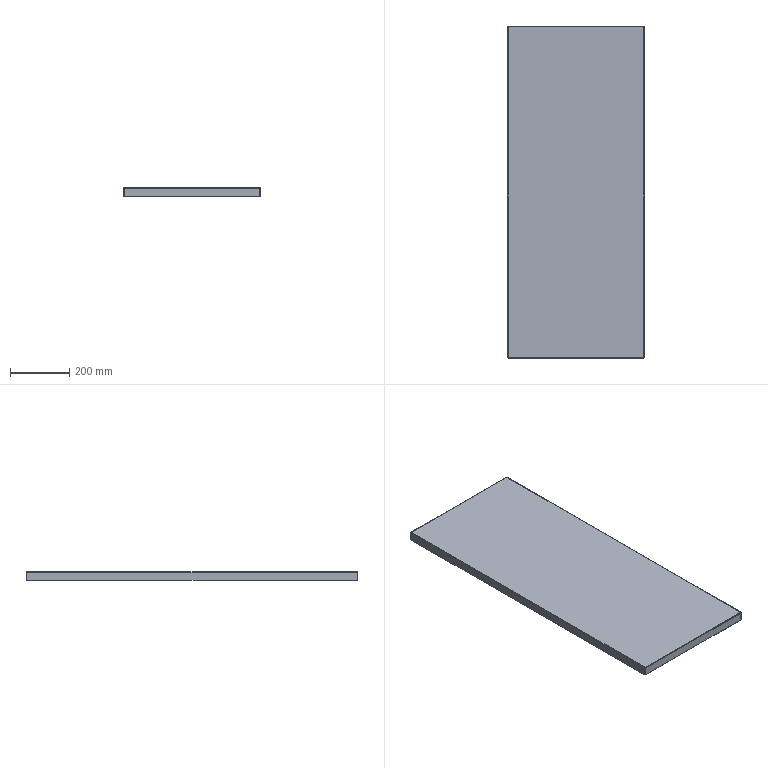Part | 1 solid | 38 faces | box 460 x 1120 x 30 mm | volume 724746 mm3 | plane 22 | spline 8 | cylinder 8 | commonest cylinder face diameters 1.465 x4 3.865 x4
STEP:
#1=CARTESIAN_POINT('',(-228.067,-558.067,-1.2));
#2=VERTEX_POINT('',#1);
#3=CARTESIAN_POINT('',(228.067,-558.067,-1.2));
#4=VERTEX_POINT('',#3);
#5=CARTESIAN_POINT('',(-228.093,-558.067,-1.2));
#6=DIRECTION('',(1.,0.,0.));
#7=VECTOR('',#6,1000.);
#8=LINE('',#5,#7);
#9=EDGE_CURVE('',#2,#4,#8,.T.);
#10=ORIENTED_EDGE('',*,*,#9,.F.);
#11=CARTESIAN_POINT('',(-228.067,558.067,-1.2));
#12=VERTEX_POINT('',#11);
#13=CARTESIAN_POINT('',(-228.067,558.093,-1.2));
#14=DIRECTION('',(0.,-1.,0.));
#15=VECTOR('',#14,1000.);
#16=LINE('',#13,#15);
#17=EDGE_CURVE('',#12,#2,#16,.T.);
#18=ORIENTED_EDGE('',*,*,#17,.F.);
#19=CARTESIAN_POINT('',(228.067,558.067,-1.2));
#20=VERTEX_POINT('',#19);
#21=CARTESIAN_POINT('',(228.093,558.067,-1.2));
#22=DIRECTION('',(-1.,0.,0.));
#23=VECTOR('',#22,1000.);
#24=LINE('',#21,#23);
#25=EDGE_CURVE('',#20,#12,#24,.T.);
#26=ORIENTED_EDGE('',*,*,#25,.F.);
#27=CARTESIAN_POINT('',(228.067,-558.093,-1.2));
#28=DIRECTION('',(0.,1.,0.));
#29=VECTOR('',#28,1000.);
#30=LINE('',#27,#29);
#31=EDGE_CURVE('',#4,#20,#30,.T.);
#32=ORIENTED_EDGE('',*,*,#31,.F.);
#33=EDGE_LOOP('',(#10,#18,#26,#32));
#34=FACE_OUTER_BOUND('',#33,.T.);
#35=CARTESIAN_POINT('',(0.,0.,-1.2));
#36=DIRECTION('',(0.,0.,1.));
#37=DIRECTION('',(1.,0.,0.));
#38=AXIS2_PLACEMENT_3D('',#35,#36,#37);
#39=PLANE('',#38);
#40=ADVANCED_FACE('',(#34),#39,.F.);
#41=CARTESIAN_POINT('',(-228.067,558.067,0.));
#42=VERTEX_POINT('',#41);
#43=CARTESIAN_POINT('',(-228.067,-558.067,0.));
#44=VERTEX_POINT('',#43);
#45=CARTESIAN_POINT('',(-228.067,558.093,0.));
#46=DIRECTION('',(0.,-1.,0.));
#47=VECTOR('',#46,1000.);
#48=LINE('',#45,#47);
#49=EDGE_CURVE('',#42,#44,#48,.T.);
#50=ORIENTED_EDGE('',*,*,#49,.T.);
#51=CARTESIAN_POINT('',(228.067,-558.067,0.));
#52=VERTEX_POINT('',#51);
#53=CARTESIAN_POINT('',(-228.093,-558.067,0.));
#54=DIRECTION('',(1.,0.,0.));
#55=VECTOR('',#54,1000.);
#56=LINE('',#53,#55);
#57=EDGE_CURVE('',#44,#52,#56,.T.);
#58=ORIENTED_EDGE('',*,*,#57,.T.);
#59=CARTESIAN_POINT('',(228.067,558.067,0.));
#60=VERTEX_POINT('',#59);
#61=CARTESIAN_POINT('',(228.067,-558.093,0.));
#62=DIRECTION('',(0.,1.,0.));
#63=VECTOR('',#62,1000.);
#64=LINE('',#61,#63);
#65=EDGE_CURVE('',#52,#60,#64,.T.);
#66=ORIENTED_EDGE('',*,*,#65,.T.);
#67=CARTESIAN_POINT('',(228.093,558.067,0.));
#68=DIRECTION('',(-1.,0.,0.));
#69=VECTOR('',#68,1000.);
#70=LINE('',#67,#69);
#71=EDGE_CURVE('',#60,#42,#70,.T.);
#72=ORIENTED_EDGE('',*,*,#71,.T.);
#73=EDGE_LOOP('',(#50,#58,#66,#72));
#74=FACE_OUTER_BOUND('',#73,.T.);
#75=CARTESIAN_POINT('',(0.,0.,0.));
#76=DIRECTION('',(0.,0.,1.));
#77=DIRECTION('',(1.,0.,0.));
#78=AXIS2_PLACEMENT_3D('',#75,#76,#77);
#79=PLANE('',#78);
#80=ADVANCED_FACE('',(#74),#79,.T.);
#81=CARTESIAN_POINT('',(-228.093,560.,-1.933));
#82=VERTEX_POINT('',#81);
#83=CARTESIAN_POINT('',(-228.093,558.8,-1.933));
#84=VERTEX_POINT('',#83);
#85=CARTESIAN_POINT('',(-228.093,558.8,-1.933));
#86=DIRECTION('',(0.,-1.,0.));
#87=VECTOR('',#86,1000.);
#88=LINE('',#85,#87);
#89=EDGE_CURVE('',#82,#84,#88,.T.);
#90=ORIENTED_EDGE('',*,*,#89,.T.);
#91=CARTESIAN_POINT('',(-228.067,558.067,-1.2));
#92=CARTESIAN_POINT('',(-228.072,558.259,-1.2));
#93=CARTESIAN_POINT('',(-228.076,558.45,-1.279));
#94=CARTESIAN_POINT('',(-228.084,558.721,-1.55));
#95=CARTESIAN_POINT('',(-228.089,558.8,-1.741));
#96=CARTESIAN_POINT('',(-228.093,558.8,-1.933));
#97=B_SPLINE_CURVE_WITH_KNOTS('',3,(#91,#92,#93,#94,#95,#96),.UNSPECIFIED.,.F.,.F.,(4,2,4),(0.,0.5,1.),.UNSPECIFIED.);
#98=EDGE_CURVE('',#12,#84,#97,.T.);
#99=ORIENTED_EDGE('',*,*,#98,.F.);
#100=CARTESIAN_POINT('',(-228.067,558.067,-1.2));
#101=DIRECTION('',(0.,0.,1.));
#102=VECTOR('',#101,1000.);
#103=LINE('',#100,#102);
#104=EDGE_CURVE('',#12,#42,#103,.T.);
#105=ORIENTED_EDGE('',*,*,#104,.T.);
#106=CARTESIAN_POINT('',(-228.067,558.067,0.));
#107=CARTESIAN_POINT('',(-228.07,558.32,0.));
#108=CARTESIAN_POINT('',(-228.072,558.573,-0.0503));
#109=CARTESIAN_POINT('',(-228.076,559.041,-0.2439));
#110=CARTESIAN_POINT('',(-228.078,559.255,-0.3872));
#111=CARTESIAN_POINT('',(-228.082,559.613,-0.7449));
#112=CARTESIAN_POINT('',(-228.084,559.756,-0.9593));
#113=CARTESIAN_POINT('',(-228.089,559.95,-1.427));
#114=CARTESIAN_POINT('',(-228.091,560.,-1.68));
#115=CARTESIAN_POINT('',(-228.093,560.,-1.933));
#116=B_SPLINE_CURVE_WITH_KNOTS('',3,(#106,#107,#108,#109,#110,#111,#112,#113,#114,#115),.UNSPECIFIED.,.F.,.F.,(4,2,2,2,4),(0.,0.25,0.5,0.75,1.),.UNSPECIFIED.);
#117=EDGE_CURVE('',#42,#82,#116,.T.);
#118=ORIENTED_EDGE('',*,*,#117,.T.);
#119=EDGE_LOOP('',(#90,#99,#105,#118));
#120=FACE_OUTER_BOUND('',#119,.T.);
#121=CARTESIAN_POINT('',(-228.067,558.067,0.012));
#122=CARTESIAN_POINT('',(-228.07,558.322,0.012));
#123=CARTESIAN_POINT('',(-228.072,558.576,-0.03861));
#124=CARTESIAN_POINT('',(-228.076,559.047,-0.2334));
#125=CARTESIAN_POINT('',(-228.078,559.262,-0.3776));
#126=CARTESIAN_POINT('',(-228.082,559.622,-0.7376));
#127=CARTESIAN_POINT('',(-228.084,559.767,-0.9533));
#128=CARTESIAN_POINT('',(-228.089,559.961,-1.424));
#129=CARTESIAN_POINT('',(-228.091,560.012,-1.678));
#130=CARTESIAN_POINT('',(-228.093,560.012,-1.933));
#131=CARTESIAN_POINT('',(-228.067,558.067,0.));
#132=CARTESIAN_POINT('',(-228.07,558.32,0.));
#133=CARTESIAN_POINT('',(-228.072,558.573,-0.0503));
#134=CARTESIAN_POINT('',(-228.076,559.041,-0.2439));
#135=CARTESIAN_POINT('',(-228.078,559.255,-0.3872));
#136=CARTESIAN_POINT('',(-228.082,559.613,-0.7449));
#137=CARTESIAN_POINT('',(-228.084,559.756,-0.9593));
#138=CARTESIAN_POINT('',(-228.089,559.95,-1.427));
#139=CARTESIAN_POINT('',(-228.091,560.,-1.68));
#140=CARTESIAN_POINT('',(-228.093,560.,-1.933));
#141=CARTESIAN_POINT('',(-228.067,558.067,-1.2));
#142=CARTESIAN_POINT('',(-228.07,558.163,-1.2));
#143=CARTESIAN_POINT('',(-228.072,558.259,-1.219));
#144=CARTESIAN_POINT('',(-228.076,558.436,-1.292));
#145=CARTESIAN_POINT('',(-228.078,558.518,-1.347));
#146=CARTESIAN_POINT('',(-228.082,558.653,-1.482));
#147=CARTESIAN_POINT('',(-228.084,558.708,-1.564));
#148=CARTESIAN_POINT('',(-228.089,558.781,-1.741));
#149=CARTESIAN_POINT('',(-228.091,558.8,-1.837));
#150=CARTESIAN_POINT('',(-228.093,558.8,-1.933));
#151=CARTESIAN_POINT('',(-228.067,558.067,-1.212));
#152=CARTESIAN_POINT('',(-228.07,558.162,-1.212));
#153=CARTESIAN_POINT('',(-228.072,558.256,-1.231));
#154=CARTESIAN_POINT('',(-228.076,558.43,-1.303));
#155=CARTESIAN_POINT('',(-228.078,558.51,-1.356));
#156=CARTESIAN_POINT('',(-228.082,558.644,-1.49));
#157=CARTESIAN_POINT('',(-228.084,558.697,-1.57));
#158=CARTESIAN_POINT('',(-228.089,558.769,-1.744));
#159=CARTESIAN_POINT('',(-228.091,558.788,-1.838));
#160=CARTESIAN_POINT('',(-228.093,558.788,-1.933));
#161=B_SPLINE_SURFACE_WITH_KNOTS('',1,3,((#121,#122,#123,#124,#125,#126,#127,#128,#129,#130),(#131,#132,#133,#134,#135,#136,#137,#138,#139,#140),(#141,#142,#143,#144,#145,#146,#147,#148,#149,#150),(#151,#152,#153,#154,#155,#156,#157,#158,#159,#160)),.UNSPECIFIED.,.F.,.F.,.F.,(2,1,1,2),(4,2,2,2,4),(-0.01,0.,1.,1.01),(0.,0.25,0.5,0.75,1.),.UNSPECIFIED.);
#162=ADVANCED_FACE('',(#120),#161,.F.);
#163=CARTESIAN_POINT('',(228.093,558.8,-1.933));
#164=VERTEX_POINT('',#163);
#165=CARTESIAN_POINT('',(228.093,558.8,-1.933));
#166=CARTESIAN_POINT('',(228.089,558.8,-1.741));
#167=CARTESIAN_POINT('',(228.084,558.721,-1.55));
#168=CARTESIAN_POINT('',(228.076,558.45,-1.279));
#169=CARTESIAN_POINT('',(228.072,558.259,-1.2));
#170=CARTESIAN_POINT('',(228.067,558.067,-1.2));
#171=B_SPLINE_CURVE_WITH_KNOTS('',3,(#165,#166,#167,#168,#169,#170),.UNSPECIFIED.,.F.,.F.,(4,2,4),(0.,0.5,1.),.UNSPECIFIED.);
#172=EDGE_CURVE('',#164,#20,#171,.T.);
#173=ORIENTED_EDGE('',*,*,#172,.F.);
#174=CARTESIAN_POINT('',(228.093,560.,-1.933));
#175=VERTEX_POINT('',#174);
#176=CARTESIAN_POINT('',(228.093,558.8,-1.933));
#177=DIRECTION('',(0.,-1.,0.));
#178=VECTOR('',#177,1000.);
#179=LINE('',#176,#178);
#180=EDGE_CURVE('',#175,#164,#179,.T.);
#181=ORIENTED_EDGE('',*,*,#180,.F.);
#182=CARTESIAN_POINT('',(228.093,560.,-1.933));
#183=CARTESIAN_POINT('',(228.091,560.,-1.68));
#184=CARTESIAN_POINT('',(228.089,559.95,-1.427));
#185=CARTESIAN_POINT('',(228.084,559.756,-0.9593));
#186=CARTESIAN_POINT('',(228.082,559.613,-0.7449));
#187=CARTESIAN_POINT('',(228.078,559.255,-0.3872));
#188=CARTESIAN_POINT('',(228.076,559.041,-0.2439));
#189=CARTESIAN_POINT('',(228.072,558.573,-0.0503));
#190=CARTESIAN_POINT('',(228.07,558.32,0.));
#191=CARTESIAN_POINT('',(228.067,558.067,0.));
#192=B_SPLINE_CURVE_WITH_KNOTS('',3,(#182,#183,#184,#185,#186,#187,#188,#189,#190,#191),.UNSPECIFIED.,.F.,.F.,(4,2,2,2,4),(0.,0.25,0.5,0.75,1.),.UNSPECIFIED.);
#193=EDGE_CURVE('',#175,#60,#192,.T.);
#194=ORIENTED_EDGE('',*,*,#193,.T.);
#195=CARTESIAN_POINT('',(228.067,558.067,-1.2));
#196=DIRECTION('',(0.,0.,1.));
#197=VECTOR('',#196,1000.);
#198=LINE('',#195,#197);
#199=EDGE_CURVE('',#20,#60,#198,.T.);
#200=ORIENTED_EDGE('',*,*,#199,.F.);
#201=EDGE_LOOP('',(#173,#181,#194,#200));
#202=FACE_OUTER_BOUND('',#201,.T.);
#203=CARTESIAN_POINT('',(228.093,560.012,-1.933));
#204=CARTESIAN_POINT('',(228.091,560.012,-1.678));
#205=CARTESIAN_POINT('',(228.089,559.961,-1.424));
#206=CARTESIAN_POINT('',(228.084,559.767,-0.9533));
#207=CARTESIAN_POINT('',(228.082,559.622,-0.7376));
#208=CARTESIAN_POINT('',(228.078,559.262,-0.3776));
#209=CARTESIAN_POINT('',(228.076,559.047,-0.2334));
#210=CARTESIAN_POINT('',(228.072,558.576,-0.03861));
#211=CARTESIAN_POINT('',(228.07,558.322,0.012));
#212=CARTESIAN_POINT('',(228.067,558.067,0.012));
#213=CARTESIAN_POINT('',(228.093,560.,-1.933));
#214=CARTESIAN_POINT('',(228.091,560.,-1.68));
#215=CARTESIAN_POINT('',(228.089,559.95,-1.427));
#216=CARTESIAN_POINT('',(228.084,559.756,-0.9593));
#217=CARTESIAN_POINT('',(228.082,559.613,-0.7449));
#218=CARTESIAN_POINT('',(228.078,559.255,-0.3872));
#219=CARTESIAN_POINT('',(228.076,559.041,-0.2439));
#220=CARTESIAN_POINT('',(228.072,558.573,-0.0503));
#221=CARTESIAN_POINT('',(228.07,558.32,0.));
#222=CARTESIAN_POINT('',(228.067,558.067,0.));
#223=CARTESIAN_POINT('',(228.093,558.8,-1.933));
#224=CARTESIAN_POINT('',(228.091,558.8,-1.837));
#225=CARTESIAN_POINT('',(228.089,558.781,-1.741));
#226=CARTESIAN_POINT('',(228.084,558.708,-1.564));
#227=CARTESIAN_POINT('',(228.082,558.653,-1.482));
#228=CARTESIAN_POINT('',(228.078,558.518,-1.347));
#229=CARTESIAN_POINT('',(228.076,558.436,-1.292));
#230=CARTESIAN_POINT('',(228.072,558.259,-1.219));
#231=CARTESIAN_POINT('',(228.07,558.163,-1.2));
#232=CARTESIAN_POINT('',(228.067,558.067,-1.2));
#233=CARTESIAN_POINT('',(228.093,558.788,-1.933));
#234=CARTESIAN_POINT('',(228.091,558.788,-1.838));
#235=CARTESIAN_POINT('',(228.089,558.769,-1.744));
#236=CARTESIAN_POINT('',(228.084,558.697,-1.57));
#237=CARTESIAN_POINT('',(228.082,558.644,-1.49));
#238=CARTESIAN_POINT('',(228.078,558.51,-1.356));
#239=CARTESIAN_POINT('',(228.076,558.43,-1.303));
#240=CARTESIAN_POINT('',(228.072,558.256,-1.231));
#241=CARTESIAN_POINT('',(228.07,558.162,-1.212));
#242=CARTESIAN_POINT('',(228.067,558.067,-1.212));
#243=B_SPLINE_SURFACE_WITH_KNOTS('',1,3,((#203,#204,#205,#206,#207,#208,#209,#210,#211,#212),(#213,#214,#215,#216,#217,#218,#219,#220,#221,#222),(#223,#224,#225,#226,#227,#228,#229,#230,#231,#232),(#233,#234,#235,#236,#237,#238,#239,#240,#241,#242)),.UNSPECIFIED.,.F.,.F.,.F.,(2,1,1,2),(4,2,2,2,4),(-0.01,0.,1.,1.01),(0.,0.25,0.5,0.75,1.),.UNSPECIFIED.);
#244=ADVANCED_FACE('',(#202),#243,.F.);
#245=ORIENTED_EDGE('',*,*,#71,.F.);
#246=ORIENTED_EDGE('',*,*,#193,.F.);
#247=CARTESIAN_POINT('',(0.,560.,-1.933));
#248=DIRECTION('',(1.,0.,0.));
#249=VECTOR('',#248,1000.);
#250=LINE('',#247,#249);
#251=EDGE_CURVE('',#82,#175,#250,.T.);
#252=ORIENTED_EDGE('',*,*,#251,.F.);
#253=ORIENTED_EDGE('',*,*,#117,.F.);
#254=EDGE_LOOP('',(#245,#246,#252,#253));
#255=FACE_OUTER_BOUND('',#254,.T.);
#256=CARTESIAN_POINT('',(228.093,558.067,-1.933));
#257=DIRECTION('',(1.,0.,0.));
#258=DIRECTION('',(0.,1.,0.));
#259=AXIS2_PLACEMENT_3D('',#256,#257,#258);
#260=CYLINDRICAL_SURFACE('',#259,1.933);
#261=ADVANCED_FACE('',(#255),#260,.T.);
#262=ORIENTED_EDGE('',*,*,#25,.T.);
#263=ORIENTED_EDGE('',*,*,#98,.T.);
#264=CARTESIAN_POINT('',(-230.,558.8,-1.933));
#265=DIRECTION('',(1.,0.,0.));
#266=VECTOR('',#265,1000.);
#267=LINE('',#264,#266);
#268=EDGE_CURVE('',#84,#164,#267,.T.);
#269=ORIENTED_EDGE('',*,*,#268,.T.);
#270=ORIENTED_EDGE('',*,*,#172,.T.);
#271=EDGE_LOOP('',(#262,#263,#269,#270));
#272=FACE_OUTER_BOUND('',#271,.T.);
#273=CARTESIAN_POINT('',(228.093,558.067,-1.933));
#274=DIRECTION('',(1.,0.,0.));
#275=DIRECTION('',(0.,1.,0.));
#276=AXIS2_PLACEMENT_3D('',#273,#274,#275);
#277=CYLINDRICAL_SURFACE('',#276,0.7326);
#278=ADVANCED_FACE('',(#272),#277,.F.);
#279=CARTESIAN_POINT('',(-228.093,558.8,-30.));
#280=VERTEX_POINT('',#279);
#281=CARTESIAN_POINT('',(-228.093,560.,-30.));
#282=VERTEX_POINT('',#281);
#283=CARTESIAN_POINT('',(-228.093,560.,-30.));
#284=DIRECTION('',(0.,1.,0.));
#285=VECTOR('',#284,1000.);
#286=LINE('',#283,#285);
#287=EDGE_CURVE('',#280,#282,#286,.T.);
#288=ORIENTED_EDGE('',*,*,#287,.F.);
#289=CARTESIAN_POINT('',(-228.093,558.8,0.));
#290=DIRECTION('',(0.,0.,-1.));
#291=VECTOR('',#290,1000.);
#292=LINE('',#289,#291);
#293=EDGE_CURVE('',#84,#280,#292,.T.);
#294=ORIENTED_EDGE('',*,*,#293,.F.);
#295=ORIENTED_EDGE('',*,*,#89,.F.);
#296=CARTESIAN_POINT('',(-228.093,560.,0.));
#297=DIRECTION('',(0.,0.,1.));
#298=VECTOR('',#297,1000.);
#299=LINE('',#296,#298);
#300=EDGE_CURVE('',#282,#82,#299,.T.);
#301=ORIENTED_EDGE('',*,*,#300,.F.);
#302=EDGE_LOOP('',(#288,#294,#295,#301));
#303=FACE_OUTER_BOUND('',#302,.T.);
#304=CARTESIAN_POINT('',(-228.093,558.8,-1.2));
#305=DIRECTION('',(-1.,0.,0.));
#306=DIRECTION('',(0.,0.,1.));
#307=AXIS2_PLACEMENT_3D('',#304,#305,#306);
#308=PLANE('',#307);
#309=ADVANCED_FACE('',(#303),#308,.T.);
#310=CARTESIAN_POINT('',(228.093,560.,-30.));
#311=VERTEX_POINT('',#310);
#312=CARTESIAN_POINT('',(228.093,560.,-1.2));
#313=DIRECTION('',(0.,0.,1.));
#314=VECTOR('',#313,1000.);
#315=LINE('',#312,#314);
#316=EDGE_CURVE('',#311,#175,#315,.T.);
#317=ORIENTED_EDGE('',*,*,#316,.F.);
#318=CARTESIAN_POINT('',(230.,560.,-30.));
#319=DIRECTION('',(1.,0.,0.));
#320=VECTOR('',#319,1000.);
#321=LINE('',#318,#320);
#322=EDGE_CURVE('',#282,#311,#321,.T.);
#323=ORIENTED_EDGE('',*,*,#322,.F.);
#324=ORIENTED_EDGE('',*,*,#300,.T.);
#325=ORIENTED_EDGE('',*,*,#251,.T.);
#326=EDGE_LOOP('',(#317,#323,#324,#325));
#327=FACE_OUTER_BOUND('',#326,.T.);
#328=CARTESIAN_POINT('',(0.,560.,0.));
#329=DIRECTION('',(0.,1.,0.));
#330=DIRECTION('',(0.,0.,-1.));
#331=AXIS2_PLACEMENT_3D('',#328,#329,#330);
#332=PLANE('',#331);
#333=ADVANCED_FACE('',(#327),#332,.T.);
#334=CARTESIAN_POINT('',(228.093,558.8,-30.));
#335=VERTEX_POINT('',#334);
#336=CARTESIAN_POINT('',(0.,558.8,-30.));
#337=DIRECTION('',(1.,0.,0.));
#338=VECTOR('',#337,1000.);
#339=LINE('',#336,#338);
#340=EDGE_CURVE('',#280,#335,#339,.T.);
#341=ORIENTED_EDGE('',*,*,#340,.T.);
#342=CARTESIAN_POINT('',(228.093,558.8,-1.2));
#343=DIRECTION('',(0.,0.,-1.));
#344=VECTOR('',#343,1000.);
#345=LINE('',#342,#344);
#346=EDGE_CURVE('',#164,#335,#345,.T.);
#347=ORIENTED_EDGE('',*,*,#346,.F.);
#348=ORIENTED_EDGE('',*,*,#268,.F.);
#349=ORIENTED_EDGE('',*,*,#293,.T.);
#350=EDGE_LOOP('',(#341,#347,#348,#349));
#351=FACE_OUTER_BOUND('',#350,.T.);
#352=CARTESIAN_POINT('',(0.,558.8,0.));
#353=DIRECTION('',(0.,1.,0.));
#354=DIRECTION('',(0.,0.,-1.));
#355=AXIS2_PLACEMENT_3D('',#352,#353,#354);
#356=PLANE('',#355);
#357=ADVANCED_FACE('',(#351),#356,.F.);
#358=CARTESIAN_POINT('',(228.093,558.8,-30.));
#359=DIRECTION('',(0.,1.,0.));
#360=VECTOR('',#359,1000.);
#361=LINE('',#358,#360);
#362=EDGE_CURVE('',#335,#311,#361,.T.);
#363=ORIENTED_EDGE('',*,*,#362,.F.);
#364=ORIENTED_EDGE('',*,*,#340,.F.);
#365=ORIENTED_EDGE('',*,*,#287,.T.);
#366=ORIENTED_EDGE('',*,*,#322,.T.);
#367=EDGE_LOOP('',(#363,#364,#365,#366));
#368=FACE_OUTER_BOUND('',#367,.T.);
#369=CARTESIAN_POINT('',(230.,560.,-30.));
#370=DIRECTION('',(0.,0.,-1.));
#371=DIRECTION('',(-1.,0.,0.));
#372=AXIS2_PLACEMENT_3D('',#369,#370,#371);
#373=PLANE('',#372);
#374=ADVANCED_FACE('',(#368),#373,.T.);
#375=ORIENTED_EDGE('',*,*,#346,.T.);
#376=ORIENTED_EDGE('',*,*,#362,.T.);
#377=ORIENTED_EDGE('',*,*,#316,.T.);
#378=ORIENTED_EDGE('',*,*,#180,.T.);
#379=EDGE_LOOP('',(#375,#376,#377,#378));
#380=FACE_OUTER_BOUND('',#379,.T.);
#381=CARTESIAN_POINT('',(228.093,558.8,-1.2));
#382=DIRECTION('',(-1.,0.,0.));
#383=DIRECTION('',(0.,0.,1.));
#384=AXIS2_PLACEMENT_3D('',#381,#382,#383);
#385=PLANE('',#384);
#386=ADVANCED_FACE('',(#380),#385,.F.);
#387=CARTESIAN_POINT('',(230.,558.093,-1.933));
#388=VERTEX_POINT('',#387);
#389=CARTESIAN_POINT('',(228.8,558.093,-1.933));
#390=VERTEX_POINT('',#389);
#391=CARTESIAN_POINT('',(228.8,558.093,-1.933));
#392=DIRECTION('',(-1.,0.,0.));
#393=VECTOR('',#392,1000.);
#394=LINE('',#391,#393);
#395=EDGE_CURVE('',#388,#390,#394,.T.);
#396=ORIENTED_EDGE('',*,*,#395,.T.);
#397=CARTESIAN_POINT('',(228.067,558.067,-1.2));
#398=CARTESIAN_POINT('',(228.259,558.072,-1.2));
#399=CARTESIAN_POINT('',(228.45,558.076,-1.279));
#400=CARTESIAN_POINT('',(228.721,558.084,-1.55));
#401=CARTESIAN_POINT('',(228.8,558.089,-1.741));
#402=CARTESIAN_POINT('',(228.8,558.093,-1.933));
#403=B_SPLINE_CURVE_WITH_KNOTS('',3,(#397,#398,#399,#400,#401,#402),.UNSPECIFIED.,.F.,.F.,(4,2,4),(0.,0.5,1.),.UNSPECIFIED.);
#404=EDGE_CURVE('',#20,#390,#403,.T.);
#405=ORIENTED_EDGE('',*,*,#404,.F.);
#406=ORIENTED_EDGE('',*,*,#199,.T.);
#407=CARTESIAN_POINT('',(228.067,558.067,0.));
#408=CARTESIAN_POINT('',(228.32,558.07,0.));
#409=CARTESIAN_POINT('',(228.573,558.072,-0.0503));
#410=CARTESIAN_POINT('',(229.041,558.076,-0.2439));
#411=CARTESIAN_POINT('',(229.255,558.078,-0.3872));
#412=CARTESIAN_POINT('',(229.613,558.082,-0.7449));
#413=CARTESIAN_POINT('',(229.756,558.084,-0.9593));
#414=CARTESIAN_POINT('',(229.95,558.089,-1.427));
#415=CARTESIAN_POINT('',(230.,558.091,-1.68));
#416=CARTESIAN_POINT('',(230.,558.093,-1.933));
#417=B_SPLINE_CURVE_WITH_KNOTS('',3,(#407,#408,#409,#410,#411,#412,#413,#414,#415,#416),.UNSPECIFIED.,.F.,.F.,(4,2,2,2,4),(0.,0.25,0.5,0.75,1.),.UNSPECIFIED.);
#418=EDGE_CURVE('',#60,#388,#417,.T.);
#419=ORIENTED_EDGE('',*,*,#418,.T.);
#420=EDGE_LOOP('',(#396,#405,#406,#419));
#421=FACE_OUTER_BOUND('',#420,.T.);
#422=CARTESIAN_POINT('',(228.067,558.067,0.012));
#423=CARTESIAN_POINT('',(228.322,558.07,0.012));
#424=CARTESIAN_POINT('',(228.576,558.072,-0.03861));
#425=CARTESIAN_POINT('',(229.047,558.076,-0.2334));
#426=CARTESIAN_POINT('',(229.262,558.078,-0.3776));
#427=CARTESIAN_POINT('',(229.622,558.082,-0.7376));
#428=CARTESIAN_POINT('',(229.767,558.084,-0.9533));
#429=CARTESIAN_POINT('',(229.961,558.089,-1.424));
#430=CARTESIAN_POINT('',(230.012,558.091,-1.678));
#431=CARTESIAN_POINT('',(230.012,558.093,-1.933));
#432=CARTESIAN_POINT('',(228.067,558.067,0.));
#433=CARTESIAN_POINT('',(228.32,558.07,0.));
#434=CARTESIAN_POINT('',(228.573,558.072,-0.0503));
#435=CARTESIAN_POINT('',(229.041,558.076,-0.2439));
#436=CARTESIAN_POINT('',(229.255,558.078,-0.3872));
#437=CARTESIAN_POINT('',(229.613,558.082,-0.7449));
#438=CARTESIAN_POINT('',(229.756,558.084,-0.9593));
#439=CARTESIAN_POINT('',(229.95,558.089,-1.427));
#440=CARTESIAN_POINT('',(230.,558.091,-1.68));
#441=CARTESIAN_POINT('',(230.,558.093,-1.933));
#442=CARTESIAN_POINT('',(228.067,558.067,-1.2));
#443=CARTESIAN_POINT('',(228.163,558.07,-1.2));
#444=CARTESIAN_POINT('',(228.259,558.072,-1.219));
#445=CARTESIAN_POINT('',(228.436,558.076,-1.292));
#446=CARTESIAN_POINT('',(228.518,558.078,-1.347));
#447=CARTESIAN_POINT('',(228.653,558.082,-1.482));
#448=CARTESIAN_POINT('',(228.708,558.084,-1.564));
#449=CARTESIAN_POINT('',(228.781,558.089,-1.741));
#450=CARTESIAN_POINT('',(228.8,558.091,-1.837));
#451=CARTESIAN_POINT('',(228.8,558.093,-1.933));
#452=CARTESIAN_POINT('',(228.067,558.067,-1.212));
#453=CARTESIAN_POINT('',(228.162,558.07,-1.212));
#454=CARTESIAN_POINT('',(228.256,558.072,-1.231));
#455=CARTESIAN_POINT('',(228.43,558.076,-1.303));
#456=CARTESIAN_POINT('',(228.51,558.078,-1.356));
#457=CARTESIAN_POINT('',(228.644,558.082,-1.49));
#458=CARTESIAN_POINT('',(228.697,558.084,-1.57));
#459=CARTESIAN_POINT('',(228.769,558.089,-1.744));
#460=CARTESIAN_POINT('',(228.788,558.091,-1.838));
#461=CARTESIAN_POINT('',(228.788,558.093,-1.933));
#462=B_SPLINE_SURFACE_WITH_KNOTS('',1,3,((#422,#423,#424,#425,#426,#427,#428,#429,#430,#431),(#432,#433,#434,#435,#436,#437,#438,#439,#440,#441),(#442,#443,#444,#445,#446,#447,#448,#449,#450,#451),(#452,#453,#454,#455,#456,#457,#458,#459,#460,#461)),.UNSPECIFIED.,.F.,.F.,.F.,(2,1,1,2),(4,2,2,2,4),(-0.01,0.,1.,1.01),(0.,0.25,0.5,0.75,1.),.UNSPECIFIED.);
#463=ADVANCED_FACE('',(#421),#462,.F.);
#464=CARTESIAN_POINT('',(228.8,-558.093,-1.933));
#465=VERTEX_POINT('',#464);
#466=CARTESIAN_POINT('',(228.8,-558.093,-1.933));
#467=CARTESIAN_POINT('',(228.8,-558.089,-1.741));
#468=CARTESIAN_POINT('',(228.721,-558.084,-1.55));
#469=CARTESIAN_POINT('',(228.45,-558.076,-1.279));
#470=CARTESIAN_POINT('',(228.259,-558.072,-1.2));
#471=CARTESIAN_POINT('',(228.067,-558.067,-1.2));
#472=B_SPLINE_CURVE_WITH_KNOTS('',3,(#466,#467,#468,#469,#470,#471),.UNSPECIFIED.,.F.,.F.,(4,2,4),(0.,0.5,1.),.UNSPECIFIED.);
#473=EDGE_CURVE('',#465,#4,#472,.T.);
#474=ORIENTED_EDGE('',*,*,#473,.F.);
#475=CARTESIAN_POINT('',(230.,-558.093,-1.933));
#476=VERTEX_POINT('',#475);
#477=CARTESIAN_POINT('',(228.8,-558.093,-1.933));
#478=DIRECTION('',(-1.,0.,0.));
#479=VECTOR('',#478,1000.);
#480=LINE('',#477,#479);
#481=EDGE_CURVE('',#476,#465,#480,.T.);
#482=ORIENTED_EDGE('',*,*,#481,.F.);
#483=CARTESIAN_POINT('',(230.,-558.093,-1.933));
#484=CARTESIAN_POINT('',(230.,-558.091,-1.68));
#485=CARTESIAN_POINT('',(229.95,-558.089,-1.427));
#486=CARTESIAN_POINT('',(229.756,-558.084,-0.9593));
#487=CARTESIAN_POINT('',(229.613,-558.082,-0.7449));
#488=CARTESIAN_POINT('',(229.255,-558.078,-0.3872));
#489=CARTESIAN_POINT('',(229.041,-558.076,-0.2439));
#490=CARTESIAN_POINT('',(228.573,-558.072,-0.0503));
#491=CARTESIAN_POINT('',(228.32,-558.07,0.));
#492=CARTESIAN_POINT('',(228.067,-558.067,0.));
#493=B_SPLINE_CURVE_WITH_KNOTS('',3,(#483,#484,#485,#486,#487,#488,#489,#490,#491,#492),.UNSPECIFIED.,.F.,.F.,(4,2,2,2,4),(0.,0.25,0.5,0.75,1.),.UNSPECIFIED.);
#494=EDGE_CURVE('',#476,#52,#493,.T.);
#495=ORIENTED_EDGE('',*,*,#494,.T.);
#496=CARTESIAN_POINT('',(228.067,-558.067,-1.2));
#497=DIRECTION('',(0.,0.,1.));
#498=VECTOR('',#497,1000.);
#499=LINE('',#496,#498);
#500=EDGE_CURVE('',#4,#52,#499,.T.);
#501=ORIENTED_EDGE('',*,*,#500,.F.);
#502=EDGE_LOOP('',(#474,#482,#495,#501));
#503=FACE_OUTER_BOUND('',#502,.T.);
#504=CARTESIAN_POINT('',(230.012,-558.093,-1.933));
#505=CARTESIAN_POINT('',(230.012,-558.091,-1.678));
#506=CARTESIAN_POINT('',(229.961,-558.089,-1.424));
#507=CARTESIAN_POINT('',(229.767,-558.084,-0.9533));
#508=CARTESIAN_POINT('',(229.622,-558.082,-0.7376));
#509=CARTESIAN_POINT('',(229.262,-558.078,-0.3776));
#510=CARTESIAN_POINT('',(229.047,-558.076,-0.2334));
#511=CARTESIAN_POINT('',(228.576,-558.072,-0.03861));
#512=CARTESIAN_POINT('',(228.322,-558.07,0.012));
#513=CARTESIAN_POINT('',(228.067,-558.067,0.012));
#514=CARTESIAN_POINT('',(230.,-558.093,-1.933));
#515=CARTESIAN_POINT('',(230.,-558.091,-1.68));
#516=CARTESIAN_POINT('',(229.95,-558.089,-1.427));
#517=CARTESIAN_POINT('',(229.756,-558.084,-0.9593));
#518=CARTESIAN_POINT('',(229.613,-558.082,-0.7449));
#519=CARTESIAN_POINT('',(229.255,-558.078,-0.3872));
#520=CARTESIAN_POINT('',(229.041,-558.076,-0.2439));
#521=CARTESIAN_POINT('',(228.573,-558.072,-0.0503));
#522=CARTESIAN_POINT('',(228.32,-558.07,0.));
#523=CARTESIAN_POINT('',(228.067,-558.067,0.));
#524=CARTESIAN_POINT('',(228.8,-558.093,-1.933));
#525=CARTESIAN_POINT('',(228.8,-558.091,-1.837));
#526=CARTESIAN_POINT('',(228.781,-558.089,-1.741));
#527=CARTESIAN_POINT('',(228.708,-558.084,-1.564));
#528=CARTESIAN_POINT('',(228.653,-558.082,-1.482));
#529=CARTESIAN_POINT('',(228.518,-558.078,-1.347));
#530=CARTESIAN_POINT('',(228.436,-558.076,-1.292));
#531=CARTESIAN_POINT('',(228.259,-558.072,-1.219));
#532=CARTESIAN_POINT('',(228.163,-558.07,-1.2));
#533=CARTESIAN_POINT('',(228.067,-558.067,-1.2));
#534=CARTESIAN_POINT('',(228.788,-558.093,-1.933));
#535=CARTESIAN_POINT('',(228.788,-558.091,-1.838));
#536=CARTESIAN_POINT('',(228.769,-558.089,-1.744));
#537=CARTESIAN_POINT('',(228.697,-558.084,-1.57));
#538=CARTESIAN_POINT('',(228.644,-558.082,-1.49));
#539=CARTESIAN_POINT('',(228.51,-558.078,-1.356));
#540=CARTESIAN_POINT('',(228.43,-558.076,-1.303));
#541=CARTESIAN_POINT('',(228.256,-558.072,-1.231));
#542=CARTESIAN_POINT('',(228.162,-558.07,-1.212));
#543=CARTESIAN_POINT('',(228.067,-558.067,-1.212));
#544=B_SPLINE_SURFACE_WITH_KNOTS('',1,3,((#504,#505,#506,#507,#508,#509,#510,#511,#512,#513),(#514,#515,#516,#517,#518,#519,#520,#521,#522,#523),(#524,#525,#526,#527,#528,#529,#530,#531,#532,#533),(#534,#535,#536,#537,#538,#539,#540,#541,#542,#543)),.UNSPECIFIED.,.F.,.F.,.F.,(2,1,1,2),(4,2,2,2,4),(-0.01,0.,1.,1.01),(0.,0.25,0.5,0.75,1.),.UNSPECIFIED.);
#545=ADVANCED_FACE('',(#503),#544,.F.);
#546=ORIENTED_EDGE('',*,*,#65,.F.);
#547=ORIENTED_EDGE('',*,*,#494,.F.);
#548=CARTESIAN_POINT('',(230.,560.,-1.933));
#549=DIRECTION('',(0.,1.,0.));
#550=VECTOR('',#549,1000.);
#551=LINE('',#548,#550);
#552=EDGE_CURVE('',#476,#388,#551,.T.);
#553=ORIENTED_EDGE('',*,*,#552,.T.);
#554=ORIENTED_EDGE('',*,*,#418,.F.);
#555=EDGE_LOOP('',(#546,#547,#553,#554));
#556=FACE_OUTER_BOUND('',#555,.T.);
#557=CARTESIAN_POINT('',(228.067,-558.093,-1.933));
#558=DIRECTION('',(0.,-1.,0.));
#559=DIRECTION('',(1.,0.,0.));
#560=AXIS2_PLACEMENT_3D('',#557,#558,#559);
#561=CYLINDRICAL_SURFACE('',#560,1.933);
#562=ADVANCED_FACE('',(#556),#561,.T.);
#563=ORIENTED_EDGE('',*,*,#31,.T.);
#564=ORIENTED_EDGE('',*,*,#404,.T.);
#565=CARTESIAN_POINT('',(228.8,560.,-1.933));
#566=DIRECTION('',(0.,-1.,0.));
#567=VECTOR('',#566,1000.);
#568=LINE('',#565,#567);
#569=EDGE_CURVE('',#390,#465,#568,.T.);
#570=ORIENTED_EDGE('',*,*,#569,.T.);
#571=ORIENTED_EDGE('',*,*,#473,.T.);
#572=EDGE_LOOP('',(#563,#564,#570,#571));
#573=FACE_OUTER_BOUND('',#572,.T.);
#574=CARTESIAN_POINT('',(228.067,-558.093,-1.933));
#575=DIRECTION('',(0.,-1.,0.));
#576=DIRECTION('',(1.,0.,0.));
#577=AXIS2_PLACEMENT_3D('',#574,#575,#576);
#578=CYLINDRICAL_SURFACE('',#577,0.7326);
#579=ADVANCED_FACE('',(#573),#578,.F.);
#580=CARTESIAN_POINT('',(228.8,558.093,-30.));
#581=VERTEX_POINT('',#580);
#582=CARTESIAN_POINT('',(230.,558.093,-30.));
#583=VERTEX_POINT('',#582);
#584=CARTESIAN_POINT('',(230.,558.093,-30.));
#585=DIRECTION('',(1.,0.,0.));
#586=VECTOR('',#585,1000.);
#587=LINE('',#584,#586);
#588=EDGE_CURVE('',#581,#583,#587,.T.);
#589=ORIENTED_EDGE('',*,*,#588,.F.);
#590=CARTESIAN_POINT('',(228.8,558.093,0.));
#591=DIRECTION('',(0.,0.,-1.));
#592=VECTOR('',#591,1000.);
#593=LINE('',#590,#592);
#594=EDGE_CURVE('',#390,#581,#593,.T.);
#595=ORIENTED_EDGE('',*,*,#594,.F.);
#596=ORIENTED_EDGE('',*,*,#395,.F.);
#597=CARTESIAN_POINT('',(230.,558.093,-1.2));
#598=DIRECTION('',(0.,0.,-1.));
#599=VECTOR('',#598,1000.);
#600=LINE('',#597,#599);
#601=EDGE_CURVE('',#388,#583,#600,.T.);
#602=ORIENTED_EDGE('',*,*,#601,.T.);
#603=EDGE_LOOP('',(#589,#595,#596,#602));
#604=FACE_OUTER_BOUND('',#603,.T.);
#605=CARTESIAN_POINT('',(228.8,558.093,-1.2));
#606=DIRECTION('',(0.,1.,0.));
#607=DIRECTION('',(0.,0.,-1.));
#608=AXIS2_PLACEMENT_3D('',#605,#606,#607);
#609=PLANE('',#608);
#610=ADVANCED_FACE('',(#604),#609,.T.);
#611=ORIENTED_EDGE('',*,*,#552,.F.);
#612=CARTESIAN_POINT('',(230.,-558.093,-30.));
#613=VERTEX_POINT('',#612);
#614=CARTESIAN_POINT('',(230.,-558.093,0.));
#615=DIRECTION('',(0.,0.,-1.));
#616=VECTOR('',#615,1000.);
#617=LINE('',#614,#616);
#618=EDGE_CURVE('',#476,#613,#617,.T.);
#619=ORIENTED_EDGE('',*,*,#618,.T.);
#620=CARTESIAN_POINT('',(230.,560.,-30.));
#621=DIRECTION('',(0.,-1.,0.));
#622=VECTOR('',#621,1000.);
#623=LINE('',#620,#622);
#624=EDGE_CURVE('',#583,#613,#623,.T.);
#625=ORIENTED_EDGE('',*,*,#624,.F.);
#626=ORIENTED_EDGE('',*,*,#601,.F.);
#627=EDGE_LOOP('',(#611,#619,#625,#626));
#628=FACE_OUTER_BOUND('',#627,.T.);
#629=CARTESIAN_POINT('',(230.,0.,0.));
#630=DIRECTION('',(-1.,0.,0.));
#631=DIRECTION('',(0.,0.,1.));
#632=AXIS2_PLACEMENT_3D('',#629,#630,#631);
#633=PLANE('',#632);
#634=ADVANCED_FACE('',(#628),#633,.F.);
#635=CARTESIAN_POINT('',(228.8,-558.093,-30.));
#636=VERTEX_POINT('',#635);
#637=CARTESIAN_POINT('',(228.8,-558.093,-1.2));
#638=DIRECTION('',(0.,0.,-1.));
#639=VECTOR('',#638,1000.);
#640=LINE('',#637,#639);
#641=EDGE_CURVE('',#465,#636,#640,.T.);
#642=ORIENTED_EDGE('',*,*,#641,.F.);
#643=ORIENTED_EDGE('',*,*,#569,.F.);
#644=ORIENTED_EDGE('',*,*,#594,.T.);
#645=CARTESIAN_POINT('',(228.8,0.,-30.));
#646=DIRECTION('',(0.,-1.,0.));
#647=VECTOR('',#646,1000.);
#648=LINE('',#645,#647);
#649=EDGE_CURVE('',#581,#636,#648,.T.);
#650=ORIENTED_EDGE('',*,*,#649,.T.);
#651=EDGE_LOOP('',(#642,#643,#644,#650));
#652=FACE_OUTER_BOUND('',#651,.T.);
#653=CARTESIAN_POINT('',(228.8,0.,0.));
#654=DIRECTION('',(-1.,0.,0.));
#655=DIRECTION('',(0.,0.,1.));
#656=AXIS2_PLACEMENT_3D('',#653,#654,#655);
#657=PLANE('',#656);
#658=ADVANCED_FACE('',(#652),#657,.T.);
#659=CARTESIAN_POINT('',(228.8,-558.093,-30.));
#660=DIRECTION('',(1.,0.,0.));
#661=VECTOR('',#660,1000.);
#662=LINE('',#659,#661);
#663=EDGE_CURVE('',#636,#613,#662,.T.);
#664=ORIENTED_EDGE('',*,*,#663,.F.);
#665=ORIENTED_EDGE('',*,*,#649,.F.);
#666=ORIENTED_EDGE('',*,*,#588,.T.);
#667=ORIENTED_EDGE('',*,*,#624,.T.);
#668=EDGE_LOOP('',(#664,#665,#666,#667));
#669=FACE_OUTER_BOUND('',#668,.T.);
#670=CARTESIAN_POINT('',(230.,560.,-30.));
#671=DIRECTION('',(0.,0.,-1.));
#672=DIRECTION('',(0.,-1.,0.));
#673=AXIS2_PLACEMENT_3D('',#670,#671,#672);
#674=PLANE('',#673);
#675=ADVANCED_FACE('',(#669),#674,.T.);
#676=ORIENTED_EDGE('',*,*,#641,.T.);
#677=ORIENTED_EDGE('',*,*,#663,.T.);
#678=ORIENTED_EDGE('',*,*,#618,.F.);
#679=ORIENTED_EDGE('',*,*,#481,.T.);
#680=EDGE_LOOP('',(#676,#677,#678,#679));
#681=FACE_OUTER_BOUND('',#680,.T.);
#682=CARTESIAN_POINT('',(228.8,-558.093,-1.2));
#683=DIRECTION('',(0.,1.,0.));
#684=DIRECTION('',(0.,0.,-1.));
#685=AXIS2_PLACEMENT_3D('',#682,#683,#684);
#686=PLANE('',#685);
#687=ADVANCED_FACE('',(#681),#686,.F.);
#688=CARTESIAN_POINT('',(-230.,-558.093,-1.933));
#689=VERTEX_POINT('',#688);
#690=CARTESIAN_POINT('',(-228.8,-558.093,-1.933));
#691=VERTEX_POINT('',#690);
#692=CARTESIAN_POINT('',(-228.8,-558.093,-1.933));
#693=DIRECTION('',(1.,0.,0.));
#694=VECTOR('',#693,1000.);
#695=LINE('',#692,#694);
#696=EDGE_CURVE('',#689,#691,#695,.T.);
#697=ORIENTED_EDGE('',*,*,#696,.T.);
#698=CARTESIAN_POINT('',(-228.067,-558.067,-1.2));
#699=CARTESIAN_POINT('',(-228.259,-558.072,-1.2));
#700=CARTESIAN_POINT('',(-228.45,-558.076,-1.279));
#701=CARTESIAN_POINT('',(-228.721,-558.084,-1.55));
#702=CARTESIAN_POINT('',(-228.8,-558.089,-1.741));
#703=CARTESIAN_POINT('',(-228.8,-558.093,-1.933));
#704=B_SPLINE_CURVE_WITH_KNOTS('',3,(#698,#699,#700,#701,#702,#703),.UNSPECIFIED.,.F.,.F.,(4,2,4),(0.,0.5,1.),.UNSPECIFIED.);
#705=EDGE_CURVE('',#2,#691,#704,.T.);
#706=ORIENTED_EDGE('',*,*,#705,.F.);
#707=CARTESIAN_POINT('',(-228.067,-558.067,-1.2));
#708=DIRECTION('',(0.,0.,1.));
#709=VECTOR('',#708,1000.);
#710=LINE('',#707,#709);
#711=EDGE_CURVE('',#2,#44,#710,.T.);
#712=ORIENTED_EDGE('',*,*,#711,.T.);
#713=CARTESIAN_POINT('',(-228.067,-558.067,0.));
#714=CARTESIAN_POINT('',(-228.32,-558.07,0.));
#715=CARTESIAN_POINT('',(-228.573,-558.072,-0.0503));
#716=CARTESIAN_POINT('',(-229.041,-558.076,-0.2439));
#717=CARTESIAN_POINT('',(-229.255,-558.078,-0.3872));
#718=CARTESIAN_POINT('',(-229.613,-558.082,-0.7449));
#719=CARTESIAN_POINT('',(-229.756,-558.084,-0.9593));
#720=CARTESIAN_POINT('',(-229.95,-558.089,-1.427));
#721=CARTESIAN_POINT('',(-230.,-558.091,-1.68));
#722=CARTESIAN_POINT('',(-230.,-558.093,-1.933));
#723=B_SPLINE_CURVE_WITH_KNOTS('',3,(#713,#714,#715,#716,#717,#718,#719,#720,#721,#722),.UNSPECIFIED.,.F.,.F.,(4,2,2,2,4),(0.,0.25,0.5,0.75,1.),.UNSPECIFIED.);
#724=EDGE_CURVE('',#44,#689,#723,.T.);
#725=ORIENTED_EDGE('',*,*,#724,.T.);
#726=EDGE_LOOP('',(#697,#706,#712,#725));
#727=FACE_OUTER_BOUND('',#726,.T.);
#728=CARTESIAN_POINT('',(-228.067,-558.067,0.012));
#729=CARTESIAN_POINT('',(-228.322,-558.07,0.012));
#730=CARTESIAN_POINT('',(-228.576,-558.072,-0.03861));
#731=CARTESIAN_POINT('',(-229.047,-558.076,-0.2334));
#732=CARTESIAN_POINT('',(-229.262,-558.078,-0.3776));
#733=CARTESIAN_POINT('',(-229.622,-558.082,-0.7376));
#734=CARTESIAN_POINT('',(-229.767,-558.084,-0.9533));
#735=CARTESIAN_POINT('',(-229.961,-558.089,-1.424));
#736=CARTESIAN_POINT('',(-230.012,-558.091,-1.678));
#737=CARTESIAN_POINT('',(-230.012,-558.093,-1.933));
#738=CARTESIAN_POINT('',(-228.067,-558.067,0.));
#739=CARTESIAN_POINT('',(-228.32,-558.07,0.));
#740=CARTESIAN_POINT('',(-228.573,-558.072,-0.0503));
#741=CARTESIAN_POINT('',(-229.041,-558.076,-0.2439));
#742=CARTESIAN_POINT('',(-229.255,-558.078,-0.3872));
#743=CARTESIAN_POINT('',(-229.613,-558.082,-0.7449));
#744=CARTESIAN_POINT('',(-229.756,-558.084,-0.9593));
#745=CARTESIAN_POINT('',(-229.95,-558.089,-1.427));
#746=CARTESIAN_POINT('',(-230.,-558.091,-1.68));
#747=CARTESIAN_POINT('',(-230.,-558.093,-1.933));
#748=CARTESIAN_POINT('',(-228.067,-558.067,-1.2));
#749=CARTESIAN_POINT('',(-228.163,-558.07,-1.2));
#750=CARTESIAN_POINT('',(-228.259,-558.072,-1.219));
#751=CARTESIAN_POINT('',(-228.436,-558.076,-1.292));
#752=CARTESIAN_POINT('',(-228.518,-558.078,-1.347));
#753=CARTESIAN_POINT('',(-228.653,-558.082,-1.482));
#754=CARTESIAN_POINT('',(-228.708,-558.084,-1.564));
#755=CARTESIAN_POINT('',(-228.781,-558.089,-1.741));
#756=CARTESIAN_POINT('',(-228.8,-558.091,-1.837));
#757=CARTESIAN_POINT('',(-228.8,-558.093,-1.933));
#758=CARTESIAN_POINT('',(-228.067,-558.067,-1.212));
#759=CARTESIAN_POINT('',(-228.162,-558.07,-1.212));
#760=CARTESIAN_POINT('',(-228.256,-558.072,-1.231));
#761=CARTESIAN_POINT('',(-228.43,-558.076,-1.303));
#762=CARTESIAN_POINT('',(-228.51,-558.078,-1.356));
#763=CARTESIAN_POINT('',(-228.644,-558.082,-1.49));
#764=CARTESIAN_POINT('',(-228.697,-558.084,-1.57));
#765=CARTESIAN_POINT('',(-228.769,-558.089,-1.744));
#766=CARTESIAN_POINT('',(-228.788,-558.091,-1.838));
#767=CARTESIAN_POINT('',(-228.788,-558.093,-1.933));
#768=B_SPLINE_SURFACE_WITH_KNOTS('',1,3,((#728,#729,#730,#731,#732,#733,#734,#735,#736,#737),(#738,#739,#740,#741,#742,#743,#744,#745,#746,#747),(#748,#749,#750,#751,#752,#753,#754,#755,#756,#757),(#758,#759,#760,#761,#762,#763,#764,#765,#766,#767)),.UNSPECIFIED.,.F.,.F.,.F.,(2,1,1,2),(4,2,2,2,4),(-0.01,0.,1.,1.01),(0.,0.25,0.5,0.75,1.),.UNSPECIFIED.);
#769=ADVANCED_FACE('',(#727),#768,.F.);
#770=CARTESIAN_POINT('',(-228.8,558.093,-1.933));
#771=VERTEX_POINT('',#770);
#772=CARTESIAN_POINT('',(-228.8,558.093,-1.933));
#773=CARTESIAN_POINT('',(-228.8,558.089,-1.741));
#774=CARTESIAN_POINT('',(-228.721,558.084,-1.55));
#775=CARTESIAN_POINT('',(-228.45,558.076,-1.279));
#776=CARTESIAN_POINT('',(-228.259,558.072,-1.2));
#777=CARTESIAN_POINT('',(-228.067,558.067,-1.2));
#778=B_SPLINE_CURVE_WITH_KNOTS('',3,(#772,#773,#774,#775,#776,#777),.UNSPECIFIED.,.F.,.F.,(4,2,4),(0.,0.5,1.),.UNSPECIFIED.);
#779=EDGE_CURVE('',#771,#12,#778,.T.);
#780=ORIENTED_EDGE('',*,*,#779,.F.);
#781=CARTESIAN_POINT('',(-230.,558.093,-1.933));
#782=VERTEX_POINT('',#781);
#783=CARTESIAN_POINT('',(-228.8,558.093,-1.933));
#784=DIRECTION('',(1.,0.,0.));
#785=VECTOR('',#784,1000.);
#786=LINE('',#783,#785);
#787=EDGE_CURVE('',#782,#771,#786,.T.);
#788=ORIENTED_EDGE('',*,*,#787,.F.);
#789=CARTESIAN_POINT('',(-230.,558.093,-1.933));
#790=CARTESIAN_POINT('',(-230.,558.091,-1.68));
#791=CARTESIAN_POINT('',(-229.95,558.089,-1.427));
#792=CARTESIAN_POINT('',(-229.756,558.084,-0.9593));
#793=CARTESIAN_POINT('',(-229.613,558.082,-0.7449));
#794=CARTESIAN_POINT('',(-229.255,558.078,-0.3872));
#795=CARTESIAN_POINT('',(-229.041,558.076,-0.2439));
#796=CARTESIAN_POINT('',(-228.573,558.072,-0.0503));
#797=CARTESIAN_POINT('',(-228.32,558.07,0.));
#798=CARTESIAN_POINT('',(-228.067,558.067,0.));
#799=B_SPLINE_CURVE_WITH_KNOTS('',3,(#789,#790,#791,#792,#793,#794,#795,#796,#797,#798),.UNSPECIFIED.,.F.,.F.,(4,2,2,2,4),(0.,0.25,0.5,0.75,1.),.UNSPECIFIED.);
#800=EDGE_CURVE('',#782,#42,#799,.T.);
#801=ORIENTED_EDGE('',*,*,#800,.T.);
#802=ORIENTED_EDGE('',*,*,#104,.F.);
#803=EDGE_LOOP('',(#780,#788,#801,#802));
#804=FACE_OUTER_BOUND('',#803,.T.);
#805=CARTESIAN_POINT('',(-230.012,558.093,-1.933));
#806=CARTESIAN_POINT('',(-230.012,558.091,-1.678));
#807=CARTESIAN_POINT('',(-229.961,558.089,-1.424));
#808=CARTESIAN_POINT('',(-229.767,558.084,-0.9533));
#809=CARTESIAN_POINT('',(-229.622,558.082,-0.7376));
#810=CARTESIAN_POINT('',(-229.262,558.078,-0.3776));
#811=CARTESIAN_POINT('',(-229.047,558.076,-0.2334));
#812=CARTESIAN_POINT('',(-228.576,558.072,-0.03861));
#813=CARTESIAN_POINT('',(-228.322,558.07,0.012));
#814=CARTESIAN_POINT('',(-228.067,558.067,0.012));
#815=CARTESIAN_POINT('',(-230.,558.093,-1.933));
#816=CARTESIAN_POINT('',(-230.,558.091,-1.68));
#817=CARTESIAN_POINT('',(-229.95,558.089,-1.427));
#818=CARTESIAN_POINT('',(-229.756,558.084,-0.9593));
#819=CARTESIAN_POINT('',(-229.613,558.082,-0.7449));
#820=CARTESIAN_POINT('',(-229.255,558.078,-0.3872));
#821=CARTESIAN_POINT('',(-229.041,558.076,-0.2439));
#822=CARTESIAN_POINT('',(-228.573,558.072,-0.0503));
#823=CARTESIAN_POINT('',(-228.32,558.07,0.));
#824=CARTESIAN_POINT('',(-228.067,558.067,0.));
#825=CARTESIAN_POINT('',(-228.8,558.093,-1.933));
#826=CARTESIAN_POINT('',(-228.8,558.091,-1.837));
#827=CARTESIAN_POINT('',(-228.781,558.089,-1.741));
#828=CARTESIAN_POINT('',(-228.708,558.084,-1.564));
#829=CARTESIAN_POINT('',(-228.653,558.082,-1.482));
#830=CARTESIAN_POINT('',(-228.518,558.078,-1.347));
#831=CARTESIAN_POINT('',(-228.436,558.076,-1.292));
#832=CARTESIAN_POINT('',(-228.259,558.072,-1.219));
#833=CARTESIAN_POINT('',(-228.163,558.07,-1.2));
#834=CARTESIAN_POINT('',(-228.067,558.067,-1.2));
#835=CARTESIAN_POINT('',(-228.788,558.093,-1.933));
#836=CARTESIAN_POINT('',(-228.788,558.091,-1.838));
#837=CARTESIAN_POINT('',(-228.769,558.089,-1.744));
#838=CARTESIAN_POINT('',(-228.697,558.084,-1.57));
#839=CARTESIAN_POINT('',(-228.644,558.082,-1.49));
#840=CARTESIAN_POINT('',(-228.51,558.078,-1.356));
#841=CARTESIAN_POINT('',(-228.43,558.076,-1.303));
#842=CARTESIAN_POINT('',(-228.256,558.072,-1.231));
#843=CARTESIAN_POINT('',(-228.162,558.07,-1.212));
#844=CARTESIAN_POINT('',(-228.067,558.067,-1.212));
#845=B_SPLINE_SURFACE_WITH_KNOTS('',1,3,((#805,#806,#807,#808,#809,#810,#811,#812,#813,#814),(#815,#816,#817,#818,#819,#820,#821,#822,#823,#824),(#825,#826,#827,#828,#829,#830,#831,#832,#833,#834),(#835,#836,#837,#838,#839,#840,#841,#842,#843,#844)),.UNSPECIFIED.,.F.,.F.,.F.,(2,1,1,2),(4,2,2,2,4),(-0.01,0.,1.,1.01),(0.,0.25,0.5,0.75,1.),.UNSPECIFIED.);
#846=ADVANCED_FACE('',(#804),#845,.F.);
#847=ORIENTED_EDGE('',*,*,#49,.F.);
#848=ORIENTED_EDGE('',*,*,#800,.F.);
#849=CARTESIAN_POINT('',(-230.,-560.,-1.933));
#850=DIRECTION('',(0.,-1.,0.));
#851=VECTOR('',#850,1000.);
#852=LINE('',#849,#851);
#853=EDGE_CURVE('',#782,#689,#852,.T.);
#854=ORIENTED_EDGE('',*,*,#853,.T.);
#855=ORIENTED_EDGE('',*,*,#724,.F.);
#856=EDGE_LOOP('',(#847,#848,#854,#855));
#857=FACE_OUTER_BOUND('',#856,.T.);
#858=CARTESIAN_POINT('',(-228.067,558.093,-1.933));
#859=DIRECTION('',(0.,1.,0.));
#860=DIRECTION('',(-1.,0.,0.));
#861=AXIS2_PLACEMENT_3D('',#858,#859,#860);
#862=CYLINDRICAL_SURFACE('',#861,1.933);
#863=ADVANCED_FACE('',(#857),#862,.T.);
#864=ORIENTED_EDGE('',*,*,#17,.T.);
#865=ORIENTED_EDGE('',*,*,#705,.T.);
#866=CARTESIAN_POINT('',(-228.8,-560.,-1.933));
#867=DIRECTION('',(0.,1.,0.));
#868=VECTOR('',#867,1000.);
#869=LINE('',#866,#868);
#870=EDGE_CURVE('',#691,#771,#869,.T.);
#871=ORIENTED_EDGE('',*,*,#870,.T.);
#872=ORIENTED_EDGE('',*,*,#779,.T.);
#873=EDGE_LOOP('',(#864,#865,#871,#872));
#874=FACE_OUTER_BOUND('',#873,.T.);
#875=CARTESIAN_POINT('',(-228.067,558.093,-1.933));
#876=DIRECTION('',(0.,1.,0.));
#877=DIRECTION('',(-1.,0.,0.));
#878=AXIS2_PLACEMENT_3D('',#875,#876,#877);
#879=CYLINDRICAL_SURFACE('',#878,0.7326);
#880=ADVANCED_FACE('',(#874),#879,.F.);
#881=CARTESIAN_POINT('',(-228.8,-558.093,-30.));
#882=VERTEX_POINT('',#881);
#883=CARTESIAN_POINT('',(-230.,-558.093,-30.));
#884=VERTEX_POINT('',#883);
#885=CARTESIAN_POINT('',(-230.,-558.093,-30.));
#886=DIRECTION('',(-1.,0.,0.));
#887=VECTOR('',#886,1000.);
#888=LINE('',#885,#887);
#889=EDGE_CURVE('',#882,#884,#888,.T.);
#890=ORIENTED_EDGE('',*,*,#889,.F.);
#891=CARTESIAN_POINT('',(-228.8,-558.093,0.));
#892=DIRECTION('',(0.,0.,-1.));
#893=VECTOR('',#892,1000.);
#894=LINE('',#891,#893);
#895=EDGE_CURVE('',#691,#882,#894,.T.);
#896=ORIENTED_EDGE('',*,*,#895,.F.);
#897=ORIENTED_EDGE('',*,*,#696,.F.);
#898=CARTESIAN_POINT('',(-230.,-558.093,-1.2));
#899=DIRECTION('',(0.,0.,-1.));
#900=VECTOR('',#899,1000.);
#901=LINE('',#898,#900);
#902=EDGE_CURVE('',#689,#884,#901,.T.);
#903=ORIENTED_EDGE('',*,*,#902,.T.);
#904=EDGE_LOOP('',(#890,#896,#897,#903));
#905=FACE_OUTER_BOUND('',#904,.T.);
#906=CARTESIAN_POINT('',(-228.8,-558.093,-1.2));
#907=DIRECTION('',(0.,-1.,0.));
#908=DIRECTION('',(0.,0.,-1.));
#909=AXIS2_PLACEMENT_3D('',#906,#907,#908);
#910=PLANE('',#909);
#911=ADVANCED_FACE('',(#905),#910,.T.);
#912=ORIENTED_EDGE('',*,*,#853,.F.);
#913=CARTESIAN_POINT('',(-230.,558.093,-30.));
#914=VERTEX_POINT('',#913);
#915=CARTESIAN_POINT('',(-230.,558.093,0.));
#916=DIRECTION('',(0.,0.,-1.));
#917=VECTOR('',#916,1000.);
#918=LINE('',#915,#917);
#919=EDGE_CURVE('',#782,#914,#918,.T.);
#920=ORIENTED_EDGE('',*,*,#919,.T.);
#921=CARTESIAN_POINT('',(-230.,-560.,-30.));
#922=DIRECTION('',(0.,1.,0.));
#923=VECTOR('',#922,1000.);
#924=LINE('',#921,#923);
#925=EDGE_CURVE('',#884,#914,#924,.T.);
#926=ORIENTED_EDGE('',*,*,#925,.F.);
#927=ORIENTED_EDGE('',*,*,#902,.F.);
#928=EDGE_LOOP('',(#912,#920,#926,#927));
#929=FACE_OUTER_BOUND('',#928,.T.);
#930=CARTESIAN_POINT('',(-230.,0.,0.));
#931=DIRECTION('',(1.,0.,0.));
#932=DIRECTION('',(0.,0.,-1.));
#933=AXIS2_PLACEMENT_3D('',#930,#931,#932);
#934=PLANE('',#933);
#935=ADVANCED_FACE('',(#929),#934,.F.);
#936=CARTESIAN_POINT('',(-228.8,558.093,-30.));
#937=VERTEX_POINT('',#936);
#938=CARTESIAN_POINT('',(-228.8,558.093,-1.2));
#939=DIRECTION('',(0.,0.,-1.));
#940=VECTOR('',#939,1000.);
#941=LINE('',#938,#940);
#942=EDGE_CURVE('',#771,#937,#941,.T.);
#943=ORIENTED_EDGE('',*,*,#942,.F.);
#944=ORIENTED_EDGE('',*,*,#870,.F.);
#945=ORIENTED_EDGE('',*,*,#895,.T.);
#946=CARTESIAN_POINT('',(-228.8,0.,-30.));
#947=DIRECTION('',(0.,1.,0.));
#948=VECTOR('',#947,1000.);
#949=LINE('',#946,#948);
#950=EDGE_CURVE('',#882,#937,#949,.T.);
#951=ORIENTED_EDGE('',*,*,#950,.T.);
#952=EDGE_LOOP('',(#943,#944,#945,#951));
#953=FACE_OUTER_BOUND('',#952,.T.);
#954=CARTESIAN_POINT('',(-228.8,0.,0.));
#955=DIRECTION('',(1.,0.,0.));
#956=DIRECTION('',(0.,0.,-1.));
#957=AXIS2_PLACEMENT_3D('',#954,#955,#956);
#958=PLANE('',#957);
#959=ADVANCED_FACE('',(#953),#958,.T.);
#960=CARTESIAN_POINT('',(-228.8,558.093,-30.));
#961=DIRECTION('',(-1.,0.,0.));
#962=VECTOR('',#961,1000.);
#963=LINE('',#960,#962);
#964=EDGE_CURVE('',#937,#914,#963,.T.);
#965=ORIENTED_EDGE('',*,*,#964,.F.);
#966=ORIENTED_EDGE('',*,*,#950,.F.);
#967=ORIENTED_EDGE('',*,*,#889,.T.);
#968=ORIENTED_EDGE('',*,*,#925,.T.);
#969=EDGE_LOOP('',(#965,#966,#967,#968));
#970=FACE_OUTER_BOUND('',#969,.T.);
#971=CARTESIAN_POINT('',(-230.,-560.,-30.));
#972=DIRECTION('',(0.,0.,-1.));
#973=DIRECTION('',(-1.,0.,0.));
#974=AXIS2_PLACEMENT_3D('',#971,#972,#973);
#975=PLANE('',#974);
#976=ADVANCED_FACE('',(#970),#975,.T.);
#977=ORIENTED_EDGE('',*,*,#942,.T.);
#978=ORIENTED_EDGE('',*,*,#964,.T.);
#979=ORIENTED_EDGE('',*,*,#919,.F.);
#980=ORIENTED_EDGE('',*,*,#787,.T.);
#981=EDGE_LOOP('',(#977,#978,#979,#980));
#982=FACE_OUTER_BOUND('',#981,.T.);
#983=CARTESIAN_POINT('',(-228.8,558.093,-1.2));
#984=DIRECTION('',(0.,-1.,0.));
#985=DIRECTION('',(0.,0.,-1.));
#986=AXIS2_PLACEMENT_3D('',#983,#984,#985);
#987=PLANE('',#986);
#988=ADVANCED_FACE('',(#982),#987,.F.);
#989=CARTESIAN_POINT('',(228.093,-560.,-1.933));
#990=VERTEX_POINT('',#989);
#991=CARTESIAN_POINT('',(228.093,-558.8,-1.933));
#992=VERTEX_POINT('',#991);
#993=CARTESIAN_POINT('',(228.093,-558.8,-1.933));
#994=DIRECTION('',(0.,1.,0.));
#995=VECTOR('',#994,1000.);
#996=LINE('',#993,#995);
#997=EDGE_CURVE('',#990,#992,#996,.T.);
#998=ORIENTED_EDGE('',*,*,#997,.T.);
#999=CARTESIAN_POINT('',(228.067,-558.067,-1.2));
#1000=CARTESIAN_POINT('',(228.072,-558.259,-1.2));
#1001=CARTESIAN_POINT('',(228.076,-558.45,-1.279));
#1002=CARTESIAN_POINT('',(228.084,-558.721,-1.55));
#1003=CARTESIAN_POINT('',(228.089,-558.8,-1.741));
#1004=CARTESIAN_POINT('',(228.093,-558.8,-1.933));
#1005=B_SPLINE_CURVE_WITH_KNOTS('',3,(#999,#1000,#1001,#1002,#1003,#1004),.UNSPECIFIED.,.F.,.F.,(4,2,4),(0.,0.5,1.),.UNSPECIFIED.);
#1006=EDGE_CURVE('',#4,#992,#1005,.T.);
#1007=ORIENTED_EDGE('',*,*,#1006,.F.);
#1008=ORIENTED_EDGE('',*,*,#500,.T.);
#1009=CARTESIAN_POINT('',(228.067,-558.067,0.));
#1010=CARTESIAN_POINT('',(228.07,-558.32,0.));
#1011=CARTESIAN_POINT('',(228.072,-558.573,-0.0503));
#1012=CARTESIAN_POINT('',(228.076,-559.041,-0.2439));
#1013=CARTESIAN_POINT('',(228.078,-559.255,-0.3872));
#1014=CARTESIAN_POINT('',(228.082,-559.613,-0.7449));
#1015=CARTESIAN_POINT('',(228.084,-559.756,-0.9593));
#1016=CARTESIAN_POINT('',(228.089,-559.95,-1.427));
#1017=CARTESIAN_POINT('',(228.091,-560.,-1.68));
#1018=CARTESIAN_POINT('',(228.093,-560.,-1.933));
#1019=B_SPLINE_CURVE_WITH_KNOTS('',3,(#1009,#1010,#1011,#1012,#1013,#1014,#1015,#1016,#1017,#1018),.UNSPECIFIED.,.F.,.F.,(4,2,2,2,4),(0.,0.25,0.5,0.75,1.),.UNSPECIFIED.);
#1020=EDGE_CURVE('',#52,#990,#1019,.T.);
#1021=ORIENTED_EDGE('',*,*,#1020,.T.);
#1022=EDGE_LOOP('',(#998,#1007,#1008,#1021));
#1023=FACE_OUTER_BOUND('',#1022,.T.);
#1024=CARTESIAN_POINT('',(228.067,-558.067,0.012));
#1025=CARTESIAN_POINT('',(228.07,-558.322,0.012));
#1026=CARTESIAN_POINT('',(228.072,-558.576,-0.03861));
#1027=CARTESIAN_POINT('',(228.076,-559.047,-0.2334));
#1028=CARTESIAN_POINT('',(228.078,-559.262,-0.3776));
#1029=CARTESIAN_POINT('',(228.082,-559.622,-0.7376));
#1030=CARTESIAN_POINT('',(228.084,-559.767,-0.9533));
#1031=CARTESIAN_POINT('',(228.089,-559.961,-1.424));
#1032=CARTESIAN_POINT('',(228.091,-560.012,-1.678));
#1033=CARTESIAN_POINT('',(228.093,-560.012,-1.933));
#1034=CARTESIAN_POINT('',(228.067,-558.067,0.));
#1035=CARTESIAN_POINT('',(228.07,-558.32,0.));
#1036=CARTESIAN_POINT('',(228.072,-558.573,-0.0503));
#1037=CARTESIAN_POINT('',(228.076,-559.041,-0.2439));
#1038=CARTESIAN_POINT('',(228.078,-559.255,-0.3872));
#1039=CARTESIAN_POINT('',(228.082,-559.613,-0.7449));
#1040=CARTESIAN_POINT('',(228.084,-559.756,-0.9593));
#1041=CARTESIAN_POINT('',(228.089,-559.95,-1.427));
#1042=CARTESIAN_POINT('',(228.091,-560.,-1.68));
#1043=CARTESIAN_POINT('',(228.093,-560.,-1.933));
#1044=CARTESIAN_POINT('',(228.067,-558.067,-1.2));
#1045=CARTESIAN_POINT('',(228.07,-558.163,-1.2));
#1046=CARTESIAN_POINT('',(228.072,-558.259,-1.219));
#1047=CARTESIAN_POINT('',(228.076,-558.436,-1.292));
#1048=CARTESIAN_POINT('',(228.078,-558.518,-1.347));
#1049=CARTESIAN_POINT('',(228.082,-558.653,-1.482));
#1050=CARTESIAN_POINT('',(228.084,-558.708,-1.564));
#1051=CARTESIAN_POINT('',(228.089,-558.781,-1.741));
#1052=CARTESIAN_POINT('',(228.091,-558.8,-1.837));
#1053=CARTESIAN_POINT('',(228.093,-558.8,-1.933));
#1054=CARTESIAN_POINT('',(228.067,-558.067,-1.212));
#1055=CARTESIAN_POINT('',(228.07,-558.162,-1.212));
#1056=CARTESIAN_POINT('',(228.072,-558.256,-1.231));
#1057=CARTESIAN_POINT('',(228.076,-558.43,-1.303));
#1058=CARTESIAN_POINT('',(228.078,-558.51,-1.356));
#1059=CARTESIAN_POINT('',(228.082,-558.644,-1.49));
#1060=CARTESIAN_POINT('',(228.084,-558.697,-1.57));
#1061=CARTESIAN_POINT('',(228.089,-558.769,-1.744));
#1062=CARTESIAN_POINT('',(228.091,-558.788,-1.838));
#1063=CARTESIAN_POINT('',(228.093,-558.788,-1.933));
#1064=B_SPLINE_SURFACE_WITH_KNOTS('',1,3,((#1024,#1025,#1026,#1027,#1028,#1029,#1030,#1031,#1032,#1033),(#1034,#1035,#1036,#1037,#1038,#1039,#1040,#1041,#1042,#1043),(#1044,#1045,#1046,#1047,#1048,#1049,#1050,#1051,#1052,#1053),(#1054,#1055,#1056,#1057,#1058,#1059,#1060,#1061,#1062,#1063)),.UNSPECIFIED.,.F.,.F.,.F.,(2,1,1,2),(4,2,2,2,4),(-0.01,0.,1.,1.01),(0.,0.25,0.5,0.75,1.),.UNSPECIFIED.);
#1065=ADVANCED_FACE('',(#1023),#1064,.F.);
#1066=CARTESIAN_POINT('',(-228.093,-558.8,-1.933));
#1067=VERTEX_POINT('',#1066);
#1068=CARTESIAN_POINT('',(-228.093,-558.8,-1.933));
#1069=CARTESIAN_POINT('',(-228.089,-558.8,-1.741));
#1070=CARTESIAN_POINT('',(-228.084,-558.721,-1.55));
#1071=CARTESIAN_POINT('',(-228.076,-558.45,-1.279));
#1072=CARTESIAN_POINT('',(-228.072,-558.259,-1.2));
#1073=CARTESIAN_POINT('',(-228.067,-558.067,-1.2));
#1074=B_SPLINE_CURVE_WITH_KNOTS('',3,(#1068,#1069,#1070,#1071,#1072,#1073),.UNSPECIFIED.,.F.,.F.,(4,2,4),(0.,0.5,1.),.UNSPECIFIED.);
#1075=EDGE_CURVE('',#1067,#2,#1074,.T.);
#1076=ORIENTED_EDGE('',*,*,#1075,.F.);
#1077=CARTESIAN_POINT('',(-228.093,-560.,-1.933));
#1078=VERTEX_POINT('',#1077);
#1079=CARTESIAN_POINT('',(-228.093,-558.8,-1.933));
#1080=DIRECTION('',(0.,1.,0.));
#1081=VECTOR('',#1080,1000.);
#1082=LINE('',#1079,#1081);
#1083=EDGE_CURVE('',#1078,#1067,#1082,.T.);
#1084=ORIENTED_EDGE('',*,*,#1083,.F.);
#1085=CARTESIAN_POINT('',(-228.093,-560.,-1.933));
#1086=CARTESIAN_POINT('',(-228.091,-560.,-1.68));
#1087=CARTESIAN_POINT('',(-228.089,-559.95,-1.427));
#1088=CARTESIAN_POINT('',(-228.084,-559.756,-0.9593));
#1089=CARTESIAN_POINT('',(-228.082,-559.613,-0.7449));
#1090=CARTESIAN_POINT('',(-228.078,-559.255,-0.3872));
#1091=CARTESIAN_POINT('',(-228.076,-559.041,-0.2439));
#1092=CARTESIAN_POINT('',(-228.072,-558.573,-0.0503));
#1093=CARTESIAN_POINT('',(-228.07,-558.32,0.));
#1094=CARTESIAN_POINT('',(-228.067,-558.067,0.));
#1095=B_SPLINE_CURVE_WITH_KNOTS('',3,(#1085,#1086,#1087,#1088,#1089,#1090,#1091,#1092,#1093,#1094),.UNSPECIFIED.,.F.,.F.,(4,2,2,2,4),(0.,0.25,0.5,0.75,1.),.UNSPECIFIED.);
#1096=EDGE_CURVE('',#1078,#44,#1095,.T.);
#1097=ORIENTED_EDGE('',*,*,#1096,.T.);
#1098=ORIENTED_EDGE('',*,*,#711,.F.);
#1099=EDGE_LOOP('',(#1076,#1084,#1097,#1098));
#1100=FACE_OUTER_BOUND('',#1099,.T.);
#1101=CARTESIAN_POINT('',(-228.093,-560.012,-1.933));
#1102=CARTESIAN_POINT('',(-228.091,-560.012,-1.678));
#1103=CARTESIAN_POINT('',(-228.089,-559.961,-1.424));
#1104=CARTESIAN_POINT('',(-228.084,-559.767,-0.9533));
#1105=CARTESIAN_POINT('',(-228.082,-559.622,-0.7376));
#1106=CARTESIAN_POINT('',(-228.078,-559.262,-0.3776));
#1107=CARTESIAN_POINT('',(-228.076,-559.047,-0.2334));
#1108=CARTESIAN_POINT('',(-228.072,-558.576,-0.03861));
#1109=CARTESIAN_POINT('',(-228.07,-558.322,0.012));
#1110=CARTESIAN_POINT('',(-228.067,-558.067,0.012));
#1111=CARTESIAN_POINT('',(-228.093,-560.,-1.933));
#1112=CARTESIAN_POINT('',(-228.091,-560.,-1.68));
#1113=CARTESIAN_POINT('',(-228.089,-559.95,-1.427));
#1114=CARTESIAN_POINT('',(-228.084,-559.756,-0.9593));
#1115=CARTESIAN_POINT('',(-228.082,-559.613,-0.7449));
#1116=CARTESIAN_POINT('',(-228.078,-559.255,-0.3872));
#1117=CARTESIAN_POINT('',(-228.076,-559.041,-0.2439));
#1118=CARTESIAN_POINT('',(-228.072,-558.573,-0.0503));
#1119=CARTESIAN_POINT('',(-228.07,-558.32,0.));
#1120=CARTESIAN_POINT('',(-228.067,-558.067,0.));
#1121=CARTESIAN_POINT('',(-228.093,-558.8,-1.933));
#1122=CARTESIAN_POINT('',(-228.091,-558.8,-1.837));
#1123=CARTESIAN_POINT('',(-228.089,-558.781,-1.741));
#1124=CARTESIAN_POINT('',(-228.084,-558.708,-1.564));
#1125=CARTESIAN_POINT('',(-228.082,-558.653,-1.482));
#1126=CARTESIAN_POINT('',(-228.078,-558.518,-1.347));
#1127=CARTESIAN_POINT('',(-228.076,-558.436,-1.292));
#1128=CARTESIAN_POINT('',(-228.072,-558.259,-1.219));
#1129=CARTESIAN_POINT('',(-228.07,-558.163,-1.2));
#1130=CARTESIAN_POINT('',(-228.067,-558.067,-1.2));
#1131=CARTESIAN_POINT('',(-228.093,-558.788,-1.933));
#1132=CARTESIAN_POINT('',(-228.091,-558.788,-1.838));
#1133=CARTESIAN_POINT('',(-228.089,-558.769,-1.744));
#1134=CARTESIAN_POINT('',(-228.084,-558.697,-1.57));
#1135=CARTESIAN_POINT('',(-228.082,-558.644,-1.49));
#1136=CARTESIAN_POINT('',(-228.078,-558.51,-1.356));
#1137=CARTESIAN_POINT('',(-228.076,-558.43,-1.303));
#1138=CARTESIAN_POINT('',(-228.072,-558.256,-1.231));
#1139=CARTESIAN_POINT('',(-228.07,-558.162,-1.212));
#1140=CARTESIAN_POINT('',(-228.067,-558.067,-1.212));
#1141=B_SPLINE_SURFACE_WITH_KNOTS('',1,3,((#1101,#1102,#1103,#1104,#1105,#1106,#1107,#1108,#1109,#1110),(#1111,#1112,#1113,#1114,#1115,#1116,#1117,#1118,#1119,#1120),(#1121,#1122,#1123,#1124,#1125,#1126,#1127,#1128,#1129,#1130),(#1131,#1132,#1133,#1134,#1135,#1136,#1137,#1138,#1139,#1140)),.UNSPECIFIED.,.F.,.F.,.F.,(2,1,1,2),(4,2,2,2,4),(-0.01,0.,1.,1.01),(0.,0.25,0.5,0.75,1.),.UNSPECIFIED.);
#1142=ADVANCED_FACE('',(#1100),#1141,.F.);
#1143=ORIENTED_EDGE('',*,*,#57,.F.);
#1144=ORIENTED_EDGE('',*,*,#1096,.F.);
#1145=CARTESIAN_POINT('',(230.,-560.,-1.933));
#1146=DIRECTION('',(1.,0.,0.));
#1147=VECTOR('',#1146,1000.);
#1148=LINE('',#1145,#1147);
#1149=EDGE_CURVE('',#1078,#990,#1148,.T.);
#1150=ORIENTED_EDGE('',*,*,#1149,.T.);
#1151=ORIENTED_EDGE('',*,*,#1020,.F.);
#1152=EDGE_LOOP('',(#1143,#1144,#1150,#1151));
#1153=FACE_OUTER_BOUND('',#1152,.T.);
#1154=CARTESIAN_POINT('',(-228.093,-558.067,-1.933));
#1155=DIRECTION('',(-1.,0.,0.));
#1156=DIRECTION('',(0.,-1.,0.));
#1157=AXIS2_PLACEMENT_3D('',#1154,#1155,#1156);
#1158=CYLINDRICAL_SURFACE('',#1157,1.933);
#1159=ADVANCED_FACE('',(#1153),#1158,.T.);
#1160=ORIENTED_EDGE('',*,*,#9,.T.);
#1161=ORIENTED_EDGE('',*,*,#1006,.T.);
#1162=CARTESIAN_POINT('',(230.,-558.8,-1.933));
#1163=DIRECTION('',(-1.,0.,0.));
#1164=VECTOR('',#1163,1000.);
#1165=LINE('',#1162,#1164);
#1166=EDGE_CURVE('',#992,#1067,#1165,.T.);
#1167=ORIENTED_EDGE('',*,*,#1166,.T.);
#1168=ORIENTED_EDGE('',*,*,#1075,.T.);
#1169=EDGE_LOOP('',(#1160,#1161,#1167,#1168));
#1170=FACE_OUTER_BOUND('',#1169,.T.);
#1171=CARTESIAN_POINT('',(-228.093,-558.067,-1.933));
#1172=DIRECTION('',(-1.,0.,0.));
#1173=DIRECTION('',(0.,-1.,0.));
#1174=AXIS2_PLACEMENT_3D('',#1171,#1172,#1173);
#1175=CYLINDRICAL_SURFACE('',#1174,0.7326);
#1176=ADVANCED_FACE('',(#1170),#1175,.F.);
#1177=CARTESIAN_POINT('',(228.093,-558.8,-30.));
#1178=VERTEX_POINT('',#1177);
#1179=CARTESIAN_POINT('',(228.093,-560.,-30.));
#1180=VERTEX_POINT('',#1179);
#1181=CARTESIAN_POINT('',(228.093,-560.,-30.));
#1182=DIRECTION('',(0.,-1.,0.));
#1183=VECTOR('',#1182,1000.);
#1184=LINE('',#1181,#1183);
#1185=EDGE_CURVE('',#1178,#1180,#1184,.T.);
#1186=ORIENTED_EDGE('',*,*,#1185,.F.);
#1187=CARTESIAN_POINT('',(228.093,-558.8,0.));
#1188=DIRECTION('',(0.,0.,-1.));
#1189=VECTOR('',#1188,1000.);
#1190=LINE('',#1187,#1189);
#1191=EDGE_CURVE('',#992,#1178,#1190,.T.);
#1192=ORIENTED_EDGE('',*,*,#1191,.F.);
#1193=ORIENTED_EDGE('',*,*,#997,.F.);
#1194=CARTESIAN_POINT('',(228.093,-560.,-1.2));
#1195=DIRECTION('',(0.,0.,-1.));
#1196=VECTOR('',#1195,1000.);
#1197=LINE('',#1194,#1196);
#1198=EDGE_CURVE('',#990,#1180,#1197,.T.);
#1199=ORIENTED_EDGE('',*,*,#1198,.T.);
#1200=EDGE_LOOP('',(#1186,#1192,#1193,#1199));
#1201=FACE_OUTER_BOUND('',#1200,.T.);
#1202=CARTESIAN_POINT('',(228.093,-558.8,-1.2));
#1203=DIRECTION('',(1.,0.,0.));
#1204=DIRECTION('',(0.,1.,0.));
#1205=AXIS2_PLACEMENT_3D('',#1202,#1203,#1204);
#1206=PLANE('',#1205);
#1207=ADVANCED_FACE('',(#1201),#1206,.T.);
#1208=ORIENTED_EDGE('',*,*,#1149,.F.);
#1209=CARTESIAN_POINT('',(-228.093,-560.,-30.));
#1210=VERTEX_POINT('',#1209);
#1211=CARTESIAN_POINT('',(-228.093,-560.,0.));
#1212=DIRECTION('',(0.,0.,-1.));
#1213=VECTOR('',#1212,1000.);
#1214=LINE('',#1211,#1213);
#1215=EDGE_CURVE('',#1078,#1210,#1214,.T.);
#1216=ORIENTED_EDGE('',*,*,#1215,.T.);
#1217=CARTESIAN_POINT('',(230.,-560.,-30.));
#1218=DIRECTION('',(-1.,0.,0.));
#1219=VECTOR('',#1218,1000.);
#1220=LINE('',#1217,#1219);
#1221=EDGE_CURVE('',#1180,#1210,#1220,.T.);
#1222=ORIENTED_EDGE('',*,*,#1221,.F.);
#1223=ORIENTED_EDGE('',*,*,#1198,.F.);
#1224=EDGE_LOOP('',(#1208,#1216,#1222,#1223));
#1225=FACE_OUTER_BOUND('',#1224,.T.);
#1226=CARTESIAN_POINT('',(0.,-560.,0.));
#1227=DIRECTION('',(0.,1.,0.));
#1228=DIRECTION('',(0.,0.,-1.));
#1229=AXIS2_PLACEMENT_3D('',#1226,#1227,#1228);
#1230=PLANE('',#1229);
#1231=ADVANCED_FACE('',(#1225),#1230,.F.);
#1232=CARTESIAN_POINT('',(-228.093,-558.8,-30.));
#1233=VERTEX_POINT('',#1232);
#1234=CARTESIAN_POINT('',(-228.093,-558.8,-1.2));
#1235=DIRECTION('',(0.,0.,-1.));
#1236=VECTOR('',#1235,1000.);
#1237=LINE('',#1234,#1236);
#1238=EDGE_CURVE('',#1067,#1233,#1237,.T.);
#1239=ORIENTED_EDGE('',*,*,#1238,.F.);
#1240=ORIENTED_EDGE('',*,*,#1166,.F.);
#1241=ORIENTED_EDGE('',*,*,#1191,.T.);
#1242=CARTESIAN_POINT('',(0.,-558.8,-30.));
#1243=DIRECTION('',(-1.,0.,0.));
#1244=VECTOR('',#1243,1000.);
#1245=LINE('',#1242,#1244);
#1246=EDGE_CURVE('',#1178,#1233,#1245,.T.);
#1247=ORIENTED_EDGE('',*,*,#1246,.T.);
#1248=EDGE_LOOP('',(#1239,#1240,#1241,#1247));
#1249=FACE_OUTER_BOUND('',#1248,.T.);
#1250=CARTESIAN_POINT('',(0.,-558.8,0.));
#1251=DIRECTION('',(0.,1.,0.));
#1252=DIRECTION('',(0.,0.,-1.));
#1253=AXIS2_PLACEMENT_3D('',#1250,#1251,#1252);
#1254=PLANE('',#1253);
#1255=ADVANCED_FACE('',(#1249),#1254,.T.);
#1256=CARTESIAN_POINT('',(-228.093,-558.8,-30.));
#1257=DIRECTION('',(0.,-1.,0.));
#1258=VECTOR('',#1257,1000.);
#1259=LINE('',#1256,#1258);
#1260=EDGE_CURVE('',#1233,#1210,#1259,.T.);
#1261=ORIENTED_EDGE('',*,*,#1260,.F.);
#1262=ORIENTED_EDGE('',*,*,#1246,.F.);
#1263=ORIENTED_EDGE('',*,*,#1185,.T.);
#1264=ORIENTED_EDGE('',*,*,#1221,.T.);
#1265=EDGE_LOOP('',(#1261,#1262,#1263,#1264));
#1266=FACE_OUTER_BOUND('',#1265,.T.);
#1267=CARTESIAN_POINT('',(230.,-560.,-30.));
#1268=DIRECTION('',(0.,0.,-1.));
#1269=DIRECTION('',(0.,-1.,0.));
#1270=AXIS2_PLACEMENT_3D('',#1267,#1268,#1269);
#1271=PLANE('',#1270);
#1272=ADVANCED_FACE('',(#1266),#1271,.T.);
#1273=ORIENTED_EDGE('',*,*,#1238,.T.);
#1274=ORIENTED_EDGE('',*,*,#1260,.T.);
#1275=ORIENTED_EDGE('',*,*,#1215,.F.);
#1276=ORIENTED_EDGE('',*,*,#1083,.T.);
#1277=EDGE_LOOP('',(#1273,#1274,#1275,#1276));
#1278=FACE_OUTER_BOUND('',#1277,.T.);
#1279=CARTESIAN_POINT('',(-228.093,-558.8,-1.2));
#1280=DIRECTION('',(1.,0.,0.));
#1281=DIRECTION('',(0.,1.,0.));
#1282=AXIS2_PLACEMENT_3D('',#1279,#1280,#1281);
#1283=PLANE('',#1282);
#1284=ADVANCED_FACE('',(#1278),#1283,.F.);
#1285=CLOSED_SHELL('',(#40,#80,#162,#244,#261,#278,#309,#333,#357,#374,#386,#463,#545,#562,#579,#610,#634,#658,#675,#687,#769,#846,#863,#880,#911,#935,#959,#976,#988,#1065,#1142,#1159,#1176,#1207,#1231,#1255,#1272,#1284));
#1286=MANIFOLD_SOLID_BREP('',#1285);
#1287=CARTESIAN_POINT('',(0.,0.,0.));
#1288=DIRECTION('',(0.,0.,1.));
#1289=DIRECTION('',(1.,0.,0.));
#1290=AXIS2_PLACEMENT_3D('',#1287,#1288,#1289);
#1291=(LENGTH_UNIT()NAMED_UNIT(*)SI_UNIT(.MILLI.,.METRE.));
#1292=UNCERTAINTY_MEASURE_WITH_UNIT(LENGTH_MEASURE(0.00001),#1291,'','');
#1293=(NAMED_UNIT(*)PLANE_ANGLE_UNIT()SI_UNIT($,.RADIAN.));
#1294=(NAMED_UNIT(*)SI_UNIT($,.STERADIAN.)SOLID_ANGLE_UNIT());
#1295=(GEOMETRIC_REPRESENTATION_CONTEXT(3)GLOBAL_UNCERTAINTY_ASSIGNED_CONTEXT((#1292))GLOBAL_UNIT_ASSIGNED_CONTEXT((#1291,#1293,#1294))REPRESENTATION_CONTEXT('',''));
#1296=ADVANCED_BREP_SHAPE_REPRESENTATION('',(#1286,#1290),#1295);